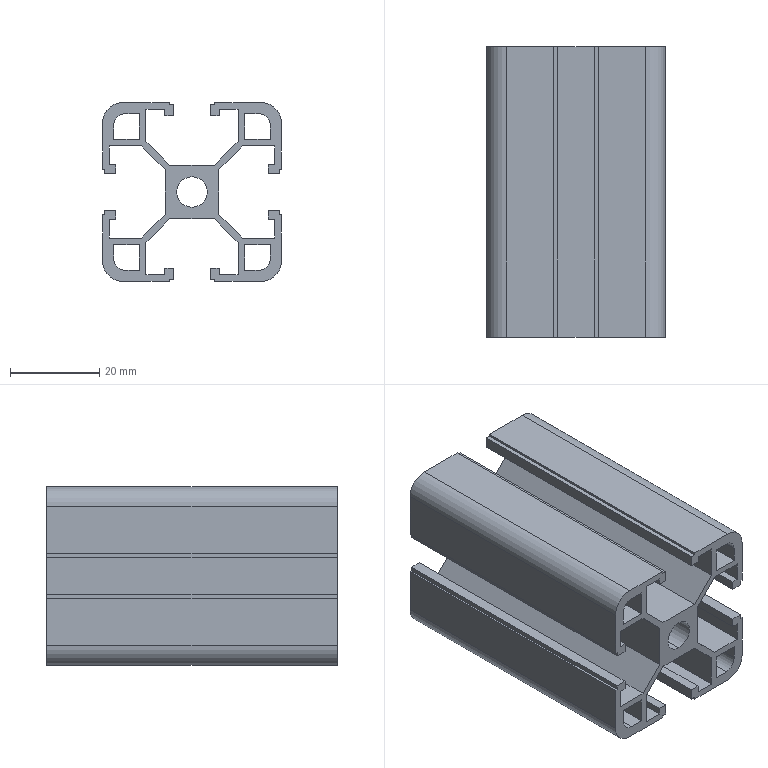Part | SolidWorks | features BaseBody 1 | 1 solid | 104 faces | box 40 x 65 x 40 mm | volume 30866 mm3 | plane 94 | cylinder 10 | commonest cylinder face diameters 5 x4 9 x4 6.8 x2